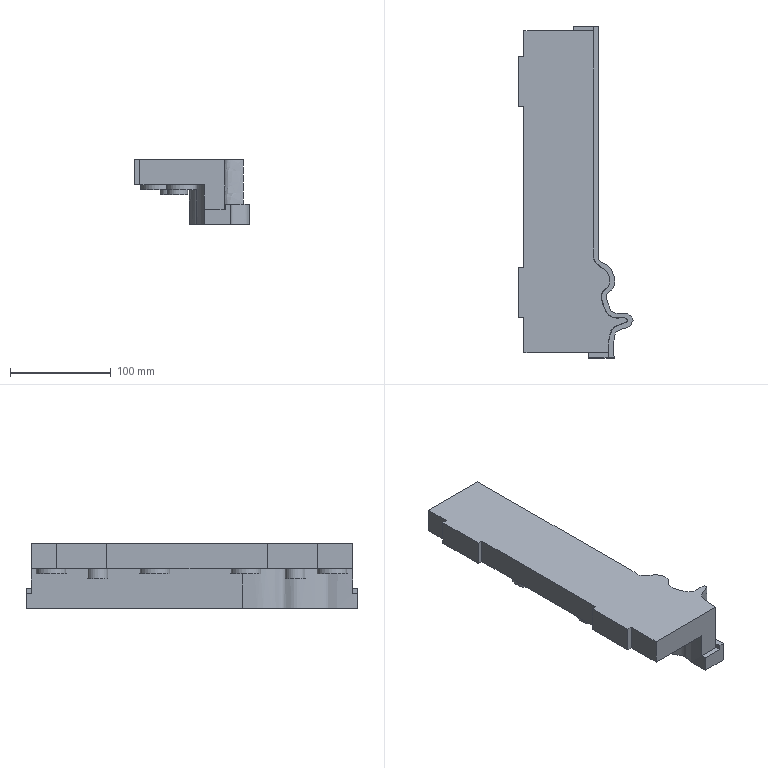Part | NX | features solid 2 | 1 solid | 42 faces | box 113.419 x 329.968 x 64.5 mm | volume 897263 mm3 | plane 27 | spline 9 | cylinder 6 | commonest cylinder face diameters 30 x4 20 x2